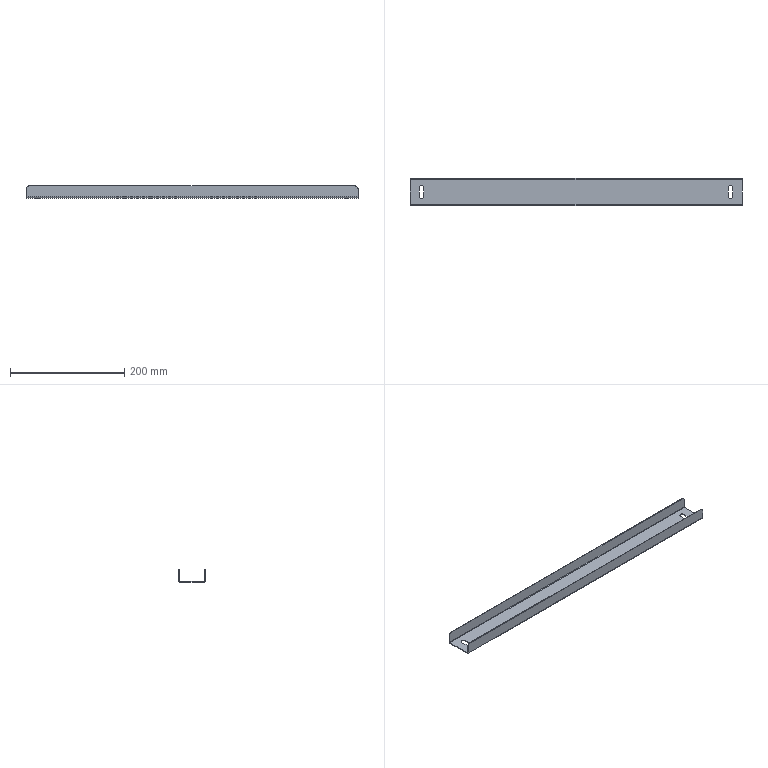Part | STEP file | PN_0040 | 1 solid | 34 faces | box 580 x 47.4 x 21.2 mm | volume 59564 mm3 | plane 22 | cylinder 12 | commonest cylinder face diameters 8.5 x4 10 x4 1.473 x2 3.873 x2